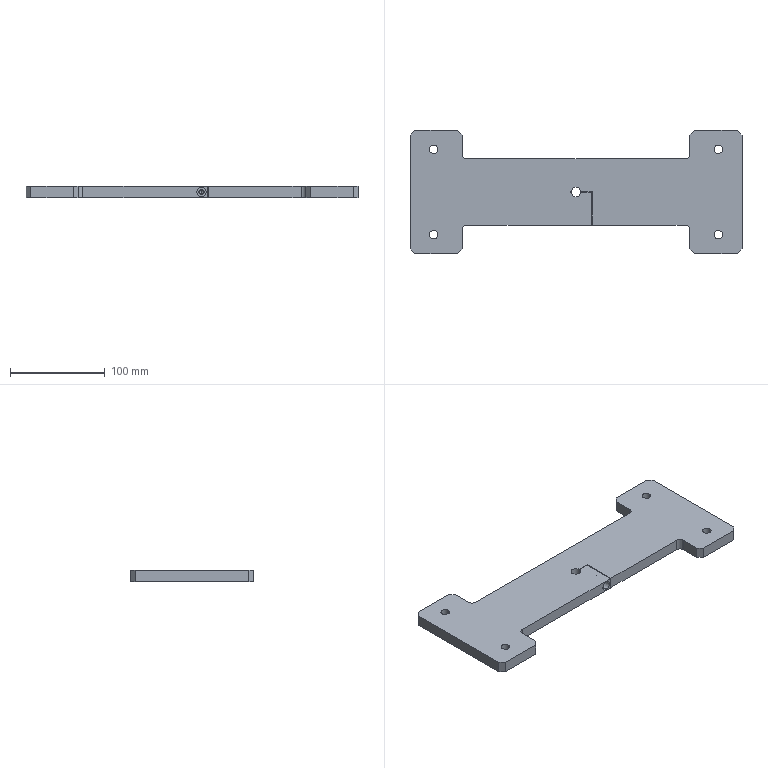Part | SolidWorks | features HoleWzd 4, ICE 4, Chamfer 1, Extrusion 1, Fillet 1 | 1 solid | 73 faces | box 350 x 130 x 12 mm | volume 363525 mm3 | plane 35 | cylinder 32 | cone 6 | commonest cylinder face diameters 9 x8 10 x8 20 x8 3.3 x4 4.2 x2 5.5 x2